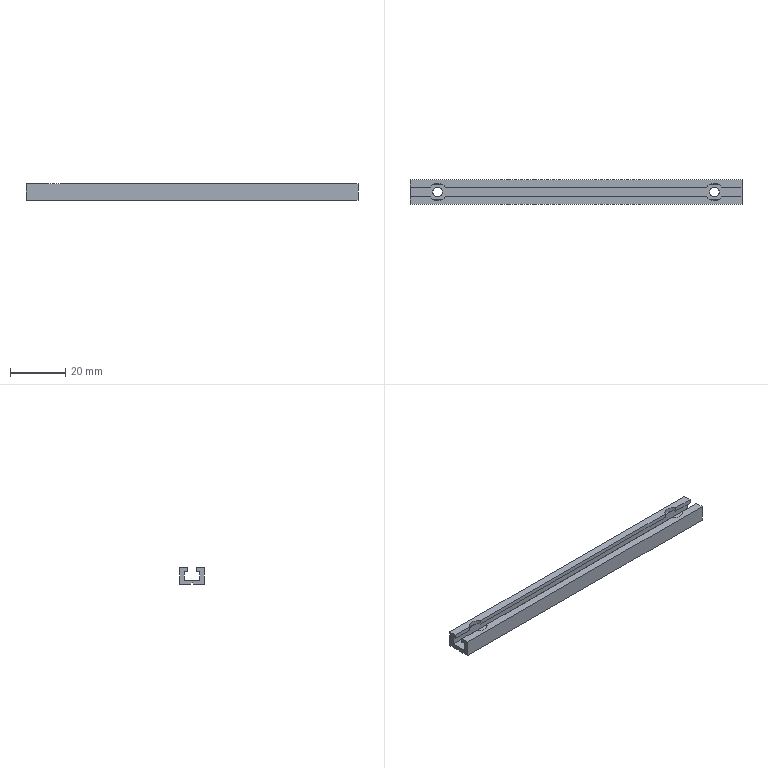Part | STEP file | 0244_013_SENAF3-120 | 1 solid | 41 faces | box 120 x 9 x 6 mm | volume 3722 mm3 | plane 33 | cylinder 8 | commonest cylinder face diameters 3.5 x4 6.5 x4